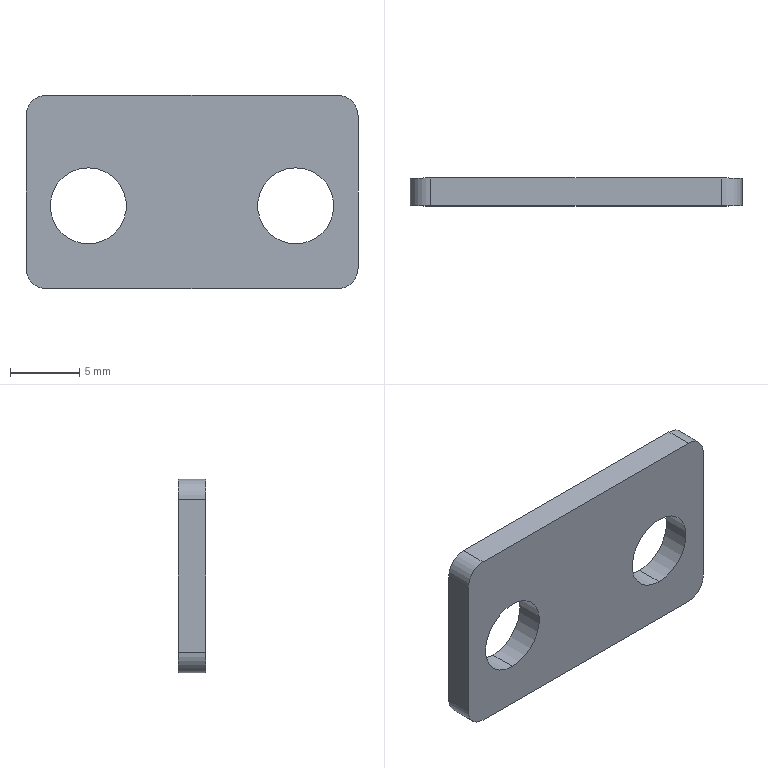Part | STEP file | 0245_011_WSHPK5 | 1 solid | 14 faces | box 24 x 2 x 14 mm | volume 573.104 mm3 | cylinder 8 | plane 6 | commonest cylinder face diameters 3 x4 5.5 x4
STEP:
#1=CARTESIAN_POINT('',(0.,0.,0.));
#2=DIRECTION('',(0.,0.,1.));
#3=DIRECTION('',(1.,0.,0.));
#4=AXIS2_PLACEMENT_3D('',#1,#2,#3);
#5=CARTESIAN_POINT('',(-7.5,2.,-10.75));
#6=VERTEX_POINT('',#5);
#7=CARTESIAN_POINT('',(-7.5,0.,-10.75));
#8=VERTEX_POINT('',#7);
#9=CARTESIAN_POINT('',(-7.5,0.,-10.75));
#10=DIRECTION('',(0.,-1.,0.));
#11=VECTOR('',#10,1.);
#12=LINE('',#9,#11);
#13=CARTESIAN_POINT('',(-7.5,0.,-8.));
#14=DIRECTION('',(0.,-1.,0.));
#15=DIRECTION('',(0.,0.,-1.));
#16=AXIS2_PLACEMENT_3D('',#13,#14,#15);
#17=CYLINDRICAL_SURFACE('',#16,2.75);
#18=CARTESIAN_POINT('',(6.283,0.));
#19=DIRECTION('',(0.,1.));
#20=VECTOR('',#19,1.);
#21=LINE('',#18,#20);
#22=(GEOMETRIC_REPRESENTATION_CONTEXT(2)PARAMETRIC_REPRESENTATION_CONTEXT()REPRESENTATION_CONTEXT('',''));
#23=DEFINITIONAL_REPRESENTATION('',(#21),#22);
#24=PCURVE('',#17,#23);
#25=CARTESIAN_POINT('',(-7.5,0.,-8.));
#26=DIRECTION('',(0.,-1.,0.));
#27=DIRECTION('',(0.,0.,-1.));
#28=AXIS2_PLACEMENT_3D('',#25,#26,#27);
#29=CYLINDRICAL_SURFACE('',#28,2.75);
#30=CARTESIAN_POINT('',(0.,0.));
#31=DIRECTION('',(0.,1.));
#32=VECTOR('',#31,1.);
#33=LINE('',#30,#32);
#34=(GEOMETRIC_REPRESENTATION_CONTEXT(2)PARAMETRIC_REPRESENTATION_CONTEXT()REPRESENTATION_CONTEXT('',''));
#35=DEFINITIONAL_REPRESENTATION('',(#33),#34);
#36=PCURVE('',#29,#35);
#37=SURFACE_CURVE('',#12,(#24,#36),.PCURVE_S1.);
#38=EDGE_CURVE('',#6,#8,#37,.T.);
#39=ORIENTED_EDGE('',*,*,#38,.T.);
#40=CARTESIAN_POINT('',(-7.5,0.,-5.25));
#41=VERTEX_POINT('',#40);
#42=CARTESIAN_POINT('',(-7.5,0.,-8.));
#43=DIRECTION('',(0.,-1.,0.));
#44=DIRECTION('',(0.,0.,-1.));
#45=AXIS2_PLACEMENT_3D('',#42,#43,#44);
#46=CIRCLE('',#45,2.75);
#47=CARTESIAN_POINT('',(0.,0.));
#48=DIRECTION('',(1.,0.));
#49=VECTOR('',#48,1.);
#50=LINE('',#47,#49);
#51=(GEOMETRIC_REPRESENTATION_CONTEXT(2)PARAMETRIC_REPRESENTATION_CONTEXT()REPRESENTATION_CONTEXT('',''));
#52=DEFINITIONAL_REPRESENTATION('',(#50),#51);
#53=PCURVE('',#17,#52);
#54=CARTESIAN_POINT('',(0.,0.,0.));
#55=DIRECTION('',(0.,1.,0.));
#56=DIRECTION('',(0.,0.,1.));
#57=AXIS2_PLACEMENT_3D('',#54,#55,#56);
#58=PLANE('',#57);
#59=CARTESIAN_POINT('',(-10.75,-7.5));
#60=CARTESIAN_POINT('',(-10.75,-2.737));
#61=CARTESIAN_POINT('',(-6.625,-5.118));
#62=CARTESIAN_POINT('',(-2.5,-7.5));
#63=CARTESIAN_POINT('',(-6.625,-9.882));
#64=CARTESIAN_POINT('',(-10.75,-12.263));
#65=CARTESIAN_POINT('',(-10.75,-7.5));
#66=(BOUNDED_CURVE()B_SPLINE_CURVE(2,(#59,#60,#61,#62,#63,#64,#65),.UNSPECIFIED.,.T.,.F.)B_SPLINE_CURVE_WITH_KNOTS((1,2,2,2,2,1),(-2.094,0.,2.094,4.189,6.283,8.378),.UNSPECIFIED.)CURVE()GEOMETRIC_REPRESENTATION_ITEM()RATIONAL_B_SPLINE_CURVE((1.,0.5,1.,0.5,1.,0.5,1.))REPRESENTATION_ITEM(''));
#67=(GEOMETRIC_REPRESENTATION_CONTEXT(2)PARAMETRIC_REPRESENTATION_CONTEXT()REPRESENTATION_CONTEXT('',''));
#68=DEFINITIONAL_REPRESENTATION('',(#66),#67);
#69=PCURVE('',#58,#68);
#70=SURFACE_CURVE('',#46,(#53,#69),.PCURVE_S1.);
#71=EDGE_CURVE('',#41,#8,#70,.T.);
#72=ORIENTED_EDGE('',*,*,#71,.F.);
#73=CARTESIAN_POINT('',(-7.5,2.,-5.25));
#74=VERTEX_POINT('',#73);
#75=CARTESIAN_POINT('',(-7.5,0.,-5.25));
#76=DIRECTION('',(0.,-1.,0.));
#77=VECTOR('',#76,1.);
#78=LINE('',#75,#77);
#79=CARTESIAN_POINT('',(3.142,0.));
#80=DIRECTION('',(0.,1.));
#81=VECTOR('',#80,1.);
#82=LINE('',#79,#81);
#83=(GEOMETRIC_REPRESENTATION_CONTEXT(2)PARAMETRIC_REPRESENTATION_CONTEXT()REPRESENTATION_CONTEXT('',''));
#84=DEFINITIONAL_REPRESENTATION('',(#82),#83);
#85=PCURVE('',#17,#84);
#86=CARTESIAN_POINT('',(3.142,0.));
#87=DIRECTION('',(0.,1.));
#88=VECTOR('',#87,1.);
#89=LINE('',#86,#88);
#90=(GEOMETRIC_REPRESENTATION_CONTEXT(2)PARAMETRIC_REPRESENTATION_CONTEXT()REPRESENTATION_CONTEXT('',''));
#91=DEFINITIONAL_REPRESENTATION('',(#89),#90);
#92=PCURVE('',#29,#91);
#93=SURFACE_CURVE('',#78,(#85,#92),.PCURVE_S1.);
#94=EDGE_CURVE('',#74,#41,#93,.T.);
#95=ORIENTED_EDGE('',*,*,#94,.F.);
#96=CARTESIAN_POINT('',(-7.5,2.,-8.));
#97=DIRECTION('',(0.,-1.,0.));
#98=DIRECTION('',(0.,0.,-1.));
#99=AXIS2_PLACEMENT_3D('',#96,#97,#98);
#100=CIRCLE('',#99,2.75);
#101=CARTESIAN_POINT('',(0.,-2.));
#102=DIRECTION('',(1.,0.));
#103=VECTOR('',#102,1.);
#104=LINE('',#101,#103);
#105=(GEOMETRIC_REPRESENTATION_CONTEXT(2)PARAMETRIC_REPRESENTATION_CONTEXT()REPRESENTATION_CONTEXT('',''));
#106=DEFINITIONAL_REPRESENTATION('',(#104),#105);
#107=PCURVE('',#17,#106);
#108=CARTESIAN_POINT('',(0.,2.,0.));
#109=DIRECTION('',(0.,1.,0.));
#110=DIRECTION('',(0.,0.,1.));
#111=AXIS2_PLACEMENT_3D('',#108,#109,#110);
#112=PLANE('',#111);
#113=CARTESIAN_POINT('',(-10.75,-7.5));
#114=CARTESIAN_POINT('',(-10.75,-2.737));
#115=CARTESIAN_POINT('',(-6.625,-5.118));
#116=CARTESIAN_POINT('',(-2.5,-7.5));
#117=CARTESIAN_POINT('',(-6.625,-9.882));
#118=CARTESIAN_POINT('',(-10.75,-12.263));
#119=CARTESIAN_POINT('',(-10.75,-7.5));
#120=(BOUNDED_CURVE()B_SPLINE_CURVE(2,(#113,#114,#115,#116,#117,#118,#119),.UNSPECIFIED.,.T.,.F.)B_SPLINE_CURVE_WITH_KNOTS((1,2,2,2,2,1),(-2.094,0.,2.094,4.189,6.283,8.378),.UNSPECIFIED.)CURVE()GEOMETRIC_REPRESENTATION_ITEM()RATIONAL_B_SPLINE_CURVE((1.,0.5,1.,0.5,1.,0.5,1.))REPRESENTATION_ITEM(''));
#121=(GEOMETRIC_REPRESENTATION_CONTEXT(2)PARAMETRIC_REPRESENTATION_CONTEXT()REPRESENTATION_CONTEXT('',''));
#122=DEFINITIONAL_REPRESENTATION('',(#120),#121);
#123=PCURVE('',#112,#122);
#124=SURFACE_CURVE('',#100,(#107,#123),.PCURVE_S1.);
#125=EDGE_CURVE('',#74,#6,#124,.T.);
#126=ORIENTED_EDGE('',*,*,#125,.T.);
#127=EDGE_LOOP('',(#39,#72,#95,#126));
#128=FACE_BOUND('',#127,.F.);
#129=ADVANCED_FACE('',(#128),#17,.F.);
#130=CARTESIAN_POINT('',(7.5,2.,-10.75));
#131=VERTEX_POINT('',#130);
#132=CARTESIAN_POINT('',(7.5,0.,-10.75));
#133=VERTEX_POINT('',#132);
#134=CARTESIAN_POINT('',(7.5,0.,-10.75));
#135=DIRECTION('',(0.,-1.,0.));
#136=VECTOR('',#135,1.);
#137=LINE('',#134,#136);
#138=CARTESIAN_POINT('',(7.5,0.,-8.));
#139=DIRECTION('',(0.,-1.,0.));
#140=DIRECTION('',(0.,0.,-1.));
#141=AXIS2_PLACEMENT_3D('',#138,#139,#140);
#142=CYLINDRICAL_SURFACE('',#141,2.75);
#143=CARTESIAN_POINT('',(6.283,0.));
#144=DIRECTION('',(0.,1.));
#145=VECTOR('',#144,1.);
#146=LINE('',#143,#145);
#147=(GEOMETRIC_REPRESENTATION_CONTEXT(2)PARAMETRIC_REPRESENTATION_CONTEXT()REPRESENTATION_CONTEXT('',''));
#148=DEFINITIONAL_REPRESENTATION('',(#146),#147);
#149=PCURVE('',#142,#148);
#150=CARTESIAN_POINT('',(7.5,0.,-8.));
#151=DIRECTION('',(0.,-1.,0.));
#152=DIRECTION('',(0.,0.,-1.));
#153=AXIS2_PLACEMENT_3D('',#150,#151,#152);
#154=CYLINDRICAL_SURFACE('',#153,2.75);
#155=CARTESIAN_POINT('',(0.,0.));
#156=DIRECTION('',(0.,1.));
#157=VECTOR('',#156,1.);
#158=LINE('',#155,#157);
#159=(GEOMETRIC_REPRESENTATION_CONTEXT(2)PARAMETRIC_REPRESENTATION_CONTEXT()REPRESENTATION_CONTEXT('',''));
#160=DEFINITIONAL_REPRESENTATION('',(#158),#159);
#161=PCURVE('',#154,#160);
#162=SURFACE_CURVE('',#137,(#149,#161),.PCURVE_S1.);
#163=EDGE_CURVE('',#131,#133,#162,.T.);
#164=ORIENTED_EDGE('',*,*,#163,.T.);
#165=CARTESIAN_POINT('',(7.5,0.,-5.25));
#166=VERTEX_POINT('',#165);
#167=CARTESIAN_POINT('',(7.5,0.,-8.));
#168=DIRECTION('',(0.,-1.,0.));
#169=DIRECTION('',(0.,0.,-1.));
#170=AXIS2_PLACEMENT_3D('',#167,#168,#169);
#171=CIRCLE('',#170,2.75);
#172=CARTESIAN_POINT('',(0.,0.));
#173=DIRECTION('',(1.,0.));
#174=VECTOR('',#173,1.);
#175=LINE('',#172,#174);
#176=(GEOMETRIC_REPRESENTATION_CONTEXT(2)PARAMETRIC_REPRESENTATION_CONTEXT()REPRESENTATION_CONTEXT('',''));
#177=DEFINITIONAL_REPRESENTATION('',(#175),#176);
#178=PCURVE('',#142,#177);
#179=CARTESIAN_POINT('',(-10.75,7.5));
#180=CARTESIAN_POINT('',(-10.75,12.263));
#181=CARTESIAN_POINT('',(-6.625,9.882));
#182=CARTESIAN_POINT('',(-2.5,7.5));
#183=CARTESIAN_POINT('',(-6.625,5.118));
#184=CARTESIAN_POINT('',(-10.75,2.737));
#185=CARTESIAN_POINT('',(-10.75,7.5));
#186=(BOUNDED_CURVE()B_SPLINE_CURVE(2,(#179,#180,#181,#182,#183,#184,#185),.UNSPECIFIED.,.T.,.F.)B_SPLINE_CURVE_WITH_KNOTS((1,2,2,2,2,1),(-2.094,0.,2.094,4.189,6.283,8.378),.UNSPECIFIED.)CURVE()GEOMETRIC_REPRESENTATION_ITEM()RATIONAL_B_SPLINE_CURVE((1.,0.5,1.,0.5,1.,0.5,1.))REPRESENTATION_ITEM(''));
#187=(GEOMETRIC_REPRESENTATION_CONTEXT(2)PARAMETRIC_REPRESENTATION_CONTEXT()REPRESENTATION_CONTEXT('',''));
#188=DEFINITIONAL_REPRESENTATION('',(#186),#187);
#189=PCURVE('',#58,#188);
#190=SURFACE_CURVE('',#171,(#178,#189),.PCURVE_S1.);
#191=EDGE_CURVE('',#166,#133,#190,.T.);
#192=ORIENTED_EDGE('',*,*,#191,.F.);
#193=CARTESIAN_POINT('',(7.5,2.,-5.25));
#194=VERTEX_POINT('',#193);
#195=CARTESIAN_POINT('',(7.5,0.,-5.25));
#196=DIRECTION('',(0.,-1.,0.));
#197=VECTOR('',#196,1.);
#198=LINE('',#195,#197);
#199=CARTESIAN_POINT('',(3.142,0.));
#200=DIRECTION('',(0.,1.));
#201=VECTOR('',#200,1.);
#202=LINE('',#199,#201);
#203=(GEOMETRIC_REPRESENTATION_CONTEXT(2)PARAMETRIC_REPRESENTATION_CONTEXT()REPRESENTATION_CONTEXT('',''));
#204=DEFINITIONAL_REPRESENTATION('',(#202),#203);
#205=PCURVE('',#142,#204);
#206=CARTESIAN_POINT('',(3.142,0.));
#207=DIRECTION('',(0.,1.));
#208=VECTOR('',#207,1.);
#209=LINE('',#206,#208);
#210=(GEOMETRIC_REPRESENTATION_CONTEXT(2)PARAMETRIC_REPRESENTATION_CONTEXT()REPRESENTATION_CONTEXT('',''));
#211=DEFINITIONAL_REPRESENTATION('',(#209),#210);
#212=PCURVE('',#154,#211);
#213=SURFACE_CURVE('',#198,(#205,#212),.PCURVE_S1.);
#214=EDGE_CURVE('',#194,#166,#213,.T.);
#215=ORIENTED_EDGE('',*,*,#214,.F.);
#216=CARTESIAN_POINT('',(7.5,2.,-8.));
#217=DIRECTION('',(0.,-1.,0.));
#218=DIRECTION('',(0.,0.,-1.));
#219=AXIS2_PLACEMENT_3D('',#216,#217,#218);
#220=CIRCLE('',#219,2.75);
#221=CARTESIAN_POINT('',(0.,-2.));
#222=DIRECTION('',(1.,0.));
#223=VECTOR('',#222,1.);
#224=LINE('',#221,#223);
#225=(GEOMETRIC_REPRESENTATION_CONTEXT(2)PARAMETRIC_REPRESENTATION_CONTEXT()REPRESENTATION_CONTEXT('',''));
#226=DEFINITIONAL_REPRESENTATION('',(#224),#225);
#227=PCURVE('',#142,#226);
#228=CARTESIAN_POINT('',(-10.75,7.5));
#229=CARTESIAN_POINT('',(-10.75,12.263));
#230=CARTESIAN_POINT('',(-6.625,9.882));
#231=CARTESIAN_POINT('',(-2.5,7.5));
#232=CARTESIAN_POINT('',(-6.625,5.118));
#233=CARTESIAN_POINT('',(-10.75,2.737));
#234=CARTESIAN_POINT('',(-10.75,7.5));
#235=(BOUNDED_CURVE()B_SPLINE_CURVE(2,(#228,#229,#230,#231,#232,#233,#234),.UNSPECIFIED.,.T.,.F.)B_SPLINE_CURVE_WITH_KNOTS((1,2,2,2,2,1),(-2.094,0.,2.094,4.189,6.283,8.378),.UNSPECIFIED.)CURVE()GEOMETRIC_REPRESENTATION_ITEM()RATIONAL_B_SPLINE_CURVE((1.,0.5,1.,0.5,1.,0.5,1.))REPRESENTATION_ITEM(''));
#236=(GEOMETRIC_REPRESENTATION_CONTEXT(2)PARAMETRIC_REPRESENTATION_CONTEXT()REPRESENTATION_CONTEXT('',''));
#237=DEFINITIONAL_REPRESENTATION('',(#235),#236);
#238=PCURVE('',#112,#237);
#239=SURFACE_CURVE('',#220,(#227,#238),.PCURVE_S1.);
#240=EDGE_CURVE('',#194,#131,#239,.T.);
#241=ORIENTED_EDGE('',*,*,#240,.T.);
#242=EDGE_LOOP('',(#164,#192,#215,#241));
#243=FACE_BOUND('',#242,.F.);
#244=ADVANCED_FACE('',(#243),#142,.F.);
#245=CARTESIAN_POINT('',(-7.5,0.,-8.));
#246=DIRECTION('',(0.,-1.,0.));
#247=DIRECTION('',(0.,0.,-1.));
#248=AXIS2_PLACEMENT_3D('',#245,#246,#247);
#249=CIRCLE('',#248,2.75);
#250=CARTESIAN_POINT('',(-10.75,-7.5));
#251=CARTESIAN_POINT('',(-10.75,-2.737));
#252=CARTESIAN_POINT('',(-6.625,-5.118));
#253=CARTESIAN_POINT('',(-2.5,-7.5));
#254=CARTESIAN_POINT('',(-6.625,-9.882));
#255=CARTESIAN_POINT('',(-10.75,-12.263));
#256=CARTESIAN_POINT('',(-10.75,-7.5));
#257=(BOUNDED_CURVE()B_SPLINE_CURVE(2,(#250,#251,#252,#253,#254,#255,#256),.UNSPECIFIED.,.T.,.F.)B_SPLINE_CURVE_WITH_KNOTS((1,2,2,2,2,1),(-2.094,0.,2.094,4.189,6.283,8.378),.UNSPECIFIED.)CURVE()GEOMETRIC_REPRESENTATION_ITEM()RATIONAL_B_SPLINE_CURVE((1.,0.5,1.,0.5,1.,0.5,1.))REPRESENTATION_ITEM(''));
#258=(GEOMETRIC_REPRESENTATION_CONTEXT(2)PARAMETRIC_REPRESENTATION_CONTEXT()REPRESENTATION_CONTEXT('',''));
#259=DEFINITIONAL_REPRESENTATION('',(#257),#258);
#260=PCURVE('',#58,#259);
#261=CARTESIAN_POINT('',(0.,0.));
#262=DIRECTION('',(1.,0.));
#263=VECTOR('',#262,1.);
#264=LINE('',#261,#263);
#265=(GEOMETRIC_REPRESENTATION_CONTEXT(2)PARAMETRIC_REPRESENTATION_CONTEXT()REPRESENTATION_CONTEXT('',''));
#266=DEFINITIONAL_REPRESENTATION('',(#264),#265);
#267=PCURVE('',#29,#266);
#268=SURFACE_CURVE('',#249,(#260,#267),.PCURVE_S1.);
#269=EDGE_CURVE('',#8,#41,#268,.T.);
#270=ORIENTED_EDGE('',*,*,#269,.F.);
#271=ORIENTED_EDGE('',*,*,#71,.F.);
#272=EDGE_LOOP('',(#270,#271));
#273=FACE_BOUND('',#272,.T.);
#274=CARTESIAN_POINT('',(7.5,0.,-8.));
#275=DIRECTION('',(0.,-1.,0.));
#276=DIRECTION('',(0.,0.,-1.));
#277=AXIS2_PLACEMENT_3D('',#274,#275,#276);
#278=CIRCLE('',#277,2.75);
#279=CARTESIAN_POINT('',(-10.75,7.5));
#280=CARTESIAN_POINT('',(-10.75,12.263));
#281=CARTESIAN_POINT('',(-6.625,9.882));
#282=CARTESIAN_POINT('',(-2.5,7.5));
#283=CARTESIAN_POINT('',(-6.625,5.118));
#284=CARTESIAN_POINT('',(-10.75,2.737));
#285=CARTESIAN_POINT('',(-10.75,7.5));
#286=(BOUNDED_CURVE()B_SPLINE_CURVE(2,(#279,#280,#281,#282,#283,#284,#285),.UNSPECIFIED.,.T.,.F.)B_SPLINE_CURVE_WITH_KNOTS((1,2,2,2,2,1),(-2.094,0.,2.094,4.189,6.283,8.378),.UNSPECIFIED.)CURVE()GEOMETRIC_REPRESENTATION_ITEM()RATIONAL_B_SPLINE_CURVE((1.,0.5,1.,0.5,1.,0.5,1.))REPRESENTATION_ITEM(''));
#287=(GEOMETRIC_REPRESENTATION_CONTEXT(2)PARAMETRIC_REPRESENTATION_CONTEXT()REPRESENTATION_CONTEXT('',''));
#288=DEFINITIONAL_REPRESENTATION('',(#286),#287);
#289=PCURVE('',#58,#288);
#290=CARTESIAN_POINT('',(0.,0.));
#291=DIRECTION('',(1.,0.));
#292=VECTOR('',#291,1.);
#293=LINE('',#290,#292);
#294=(GEOMETRIC_REPRESENTATION_CONTEXT(2)PARAMETRIC_REPRESENTATION_CONTEXT()REPRESENTATION_CONTEXT('',''));
#295=DEFINITIONAL_REPRESENTATION('',(#293),#294);
#296=PCURVE('',#154,#295);
#297=SURFACE_CURVE('',#278,(#289,#296),.PCURVE_S1.);
#298=EDGE_CURVE('',#133,#166,#297,.T.);
#299=ORIENTED_EDGE('',*,*,#298,.F.);
#300=ORIENTED_EDGE('',*,*,#191,.F.);
#301=EDGE_LOOP('',(#299,#300));
#302=FACE_BOUND('',#301,.T.);
#303=CARTESIAN_POINT('',(-10.5,0.,-14.));
#304=VERTEX_POINT('',#303);
#305=CARTESIAN_POINT('',(-12.,0.,-12.5));
#306=VERTEX_POINT('',#305);
#307=CARTESIAN_POINT('',(-10.5,0.,-12.5));
#308=DIRECTION('',(0.,1.,0.));
#309=DIRECTION('',(0.,0.,-1.));
#310=AXIS2_PLACEMENT_3D('',#307,#308,#309);
#311=CIRCLE('',#310,1.5);
#312=CARTESIAN_POINT('',(-12.5,-10.5));
#313=DIRECTION('',(-1.,0.));
#314=AXIS2_PLACEMENT_2D('',#312,#313);
#315=CIRCLE('',#314,1.5);
#316=(GEOMETRIC_REPRESENTATION_CONTEXT(2)PARAMETRIC_REPRESENTATION_CONTEXT()REPRESENTATION_CONTEXT('',''));
#317=DEFINITIONAL_REPRESENTATION('',(#315),#316);
#318=PCURVE('',#58,#317);
#319=CARTESIAN_POINT('',(-10.5,0.,-12.5));
#320=DIRECTION('',(0.,-1.,0.));
#321=DIRECTION('',(0.,0.,-1.));
#322=AXIS2_PLACEMENT_3D('',#319,#320,#321);
#323=CYLINDRICAL_SURFACE('',#322,1.5);
#324=CARTESIAN_POINT('',(6.283,0.));
#325=DIRECTION('',(-1.,0.));
#326=VECTOR('',#325,1.);
#327=LINE('',#324,#326);
#328=(GEOMETRIC_REPRESENTATION_CONTEXT(2)PARAMETRIC_REPRESENTATION_CONTEXT()REPRESENTATION_CONTEXT('',''));
#329=DEFINITIONAL_REPRESENTATION('',(#327),#328);
#330=PCURVE('',#323,#329);
#331=SURFACE_CURVE('',#311,(#318,#330),.PCURVE_S1.);
#332=EDGE_CURVE('',#304,#306,#331,.T.);
#333=ORIENTED_EDGE('',*,*,#332,.F.);
#334=CARTESIAN_POINT('',(10.5,0.,-14.));
#335=VERTEX_POINT('',#334);
#336=CARTESIAN_POINT('',(0.,0.,-14.));
#337=DIRECTION('',(-1.,0.,0.));
#338=VECTOR('',#337,1.);
#339=LINE('',#336,#338);
#340=CARTESIAN_POINT('',(-14.,0.));
#341=DIRECTION('',(0.,-1.));
#342=VECTOR('',#341,1.);
#343=LINE('',#340,#342);
#344=(GEOMETRIC_REPRESENTATION_CONTEXT(2)PARAMETRIC_REPRESENTATION_CONTEXT()REPRESENTATION_CONTEXT('',''));
#345=DEFINITIONAL_REPRESENTATION('',(#343),#344);
#346=PCURVE('',#58,#345);
#347=CARTESIAN_POINT('',(-10.5,0.,-14.));
#348=DIRECTION('',(0.,0.,-1.));
#349=DIRECTION('',(-1.,0.,0.));
#350=AXIS2_PLACEMENT_3D('',#347,#348,#349);
#351=PLANE('',#350);
#352=CARTESIAN_POINT('',(-10.5,0.));
#353=DIRECTION('',(1.,0.));
#354=VECTOR('',#353,1.);
#355=LINE('',#352,#354);
#356=(GEOMETRIC_REPRESENTATION_CONTEXT(2)PARAMETRIC_REPRESENTATION_CONTEXT()REPRESENTATION_CONTEXT('',''));
#357=DEFINITIONAL_REPRESENTATION('',(#355),#356);
#358=PCURVE('',#351,#357);
#359=SURFACE_CURVE('',#339,(#346,#358),.PCURVE_S1.);
#360=EDGE_CURVE('',#335,#304,#359,.T.);
#361=ORIENTED_EDGE('',*,*,#360,.F.);
#362=CARTESIAN_POINT('',(12.,0.,-12.5));
#363=VERTEX_POINT('',#362);
#364=CARTESIAN_POINT('',(10.5,0.,-12.5));
#365=DIRECTION('',(0.,1.,0.));
#366=DIRECTION('',(0.,0.,-1.));
#367=AXIS2_PLACEMENT_3D('',#364,#365,#366);
#368=CIRCLE('',#367,1.5);
#369=CARTESIAN_POINT('',(-12.5,10.5));
#370=DIRECTION('',(-1.,0.));
#371=AXIS2_PLACEMENT_2D('',#369,#370);
#372=CIRCLE('',#371,1.5);
#373=(GEOMETRIC_REPRESENTATION_CONTEXT(2)PARAMETRIC_REPRESENTATION_CONTEXT()REPRESENTATION_CONTEXT('',''));
#374=DEFINITIONAL_REPRESENTATION('',(#372),#373);
#375=PCURVE('',#58,#374);
#376=CARTESIAN_POINT('',(10.5,0.,-12.5));
#377=DIRECTION('',(0.,-1.,0.));
#378=DIRECTION('',(0.,0.,-1.));
#379=AXIS2_PLACEMENT_3D('',#376,#377,#378);
#380=CYLINDRICAL_SURFACE('',#379,1.5);
#381=CARTESIAN_POINT('',(6.283,0.));
#382=DIRECTION('',(-1.,0.));
#383=VECTOR('',#382,1.);
#384=LINE('',#381,#383);
#385=(GEOMETRIC_REPRESENTATION_CONTEXT(2)PARAMETRIC_REPRESENTATION_CONTEXT()REPRESENTATION_CONTEXT('',''));
#386=DEFINITIONAL_REPRESENTATION('',(#384),#385);
#387=PCURVE('',#380,#386);
#388=SURFACE_CURVE('',#368,(#375,#387),.PCURVE_S1.);
#389=EDGE_CURVE('',#363,#335,#388,.T.);
#390=ORIENTED_EDGE('',*,*,#389,.F.);
#391=CARTESIAN_POINT('',(12.,0.,-1.5));
#392=VERTEX_POINT('',#391);
#393=CARTESIAN_POINT('',(12.,0.,0.));
#394=DIRECTION('',(0.,0.,-1.));
#395=VECTOR('',#394,1.);
#396=LINE('',#393,#395);
#397=CARTESIAN_POINT('',(0.,12.));
#398=DIRECTION('',(-1.,0.));
#399=VECTOR('',#398,1.);
#400=LINE('',#397,#399);
#401=(GEOMETRIC_REPRESENTATION_CONTEXT(2)PARAMETRIC_REPRESENTATION_CONTEXT()REPRESENTATION_CONTEXT('',''));
#402=DEFINITIONAL_REPRESENTATION('',(#400),#401);
#403=PCURVE('',#58,#402);
#404=CARTESIAN_POINT('',(12.,0.,-12.5));
#405=DIRECTION('',(1.,0.,0.));
#406=DIRECTION('',(0.,0.,-1.));
#407=AXIS2_PLACEMENT_3D('',#404,#405,#406);
#408=PLANE('',#407);
#409=CARTESIAN_POINT('',(-12.5,0.));
#410=DIRECTION('',(1.,0.));
#411=VECTOR('',#410,1.);
#412=LINE('',#409,#411);
#413=(GEOMETRIC_REPRESENTATION_CONTEXT(2)PARAMETRIC_REPRESENTATION_CONTEXT()REPRESENTATION_CONTEXT('',''));
#414=DEFINITIONAL_REPRESENTATION('',(#412),#413);
#415=PCURVE('',#408,#414);
#416=SURFACE_CURVE('',#396,(#403,#415),.PCURVE_S1.);
#417=EDGE_CURVE('',#392,#363,#416,.T.);
#418=ORIENTED_EDGE('',*,*,#417,.F.);
#419=CARTESIAN_POINT('',(10.5,0.,0.));
#420=VERTEX_POINT('',#419);
#421=CARTESIAN_POINT('',(10.5,0.,-1.5));
#422=DIRECTION('',(0.,1.,0.));
#423=DIRECTION('',(0.,0.,-1.));
#424=AXIS2_PLACEMENT_3D('',#421,#422,#423);
#425=CIRCLE('',#424,1.5);
#426=CARTESIAN_POINT('',(-1.5,10.5));
#427=DIRECTION('',(-1.,0.));
#428=AXIS2_PLACEMENT_2D('',#426,#427);
#429=CIRCLE('',#428,1.5);
#430=(GEOMETRIC_REPRESENTATION_CONTEXT(2)PARAMETRIC_REPRESENTATION_CONTEXT()REPRESENTATION_CONTEXT('',''));
#431=DEFINITIONAL_REPRESENTATION('',(#429),#430);
#432=PCURVE('',#58,#431);
#433=CARTESIAN_POINT('',(10.5,0.,-1.5));
#434=DIRECTION('',(0.,-1.,0.));
#435=DIRECTION('',(0.,0.,-1.));
#436=AXIS2_PLACEMENT_3D('',#433,#434,#435);
#437=CYLINDRICAL_SURFACE('',#436,1.5);
#438=CARTESIAN_POINT('',(6.283,0.));
#439=DIRECTION('',(-1.,0.));
#440=VECTOR('',#439,1.);
#441=LINE('',#438,#440);
#442=(GEOMETRIC_REPRESENTATION_CONTEXT(2)PARAMETRIC_REPRESENTATION_CONTEXT()REPRESENTATION_CONTEXT('',''));
#443=DEFINITIONAL_REPRESENTATION('',(#441),#442);
#444=PCURVE('',#437,#443);
#445=SURFACE_CURVE('',#425,(#432,#444),.PCURVE_S1.);
#446=EDGE_CURVE('',#420,#392,#445,.T.);
#447=ORIENTED_EDGE('',*,*,#446,.F.);
#448=CARTESIAN_POINT('',(-10.5,0.,0.));
#449=VERTEX_POINT('',#448);
#450=CARTESIAN_POINT('',(0.,0.,0.));
#451=DIRECTION('',(1.,0.,0.));
#452=VECTOR('',#451,1.);
#453=LINE('',#450,#452);
#454=CARTESIAN_POINT('',(0.,0.));
#455=DIRECTION('',(0.,1.));
#456=VECTOR('',#455,1.);
#457=LINE('',#454,#456);
#458=(GEOMETRIC_REPRESENTATION_CONTEXT(2)PARAMETRIC_REPRESENTATION_CONTEXT()REPRESENTATION_CONTEXT('',''));
#459=DEFINITIONAL_REPRESENTATION('',(#457),#458);
#460=PCURVE('',#58,#459);
#461=CARTESIAN_POINT('',(10.5,0.,0.));
#462=DIRECTION('',(0.,0.,1.));
#463=DIRECTION('',(1.,0.,0.));
#464=AXIS2_PLACEMENT_3D('',#461,#462,#463);
#465=PLANE('',#464);
#466=CARTESIAN_POINT('',(-10.5,0.));
#467=DIRECTION('',(1.,0.));
#468=VECTOR('',#467,1.);
#469=LINE('',#466,#468);
#470=(GEOMETRIC_REPRESENTATION_CONTEXT(2)PARAMETRIC_REPRESENTATION_CONTEXT()REPRESENTATION_CONTEXT('',''));
#471=DEFINITIONAL_REPRESENTATION('',(#469),#470);
#472=PCURVE('',#465,#471);
#473=SURFACE_CURVE('',#453,(#460,#472),.PCURVE_S1.);
#474=EDGE_CURVE('',#449,#420,#473,.T.);
#475=ORIENTED_EDGE('',*,*,#474,.F.);
#476=CARTESIAN_POINT('',(-12.,0.,-1.5));
#477=VERTEX_POINT('',#476);
#478=CARTESIAN_POINT('',(-10.5,0.,-1.5));
#479=DIRECTION('',(0.,1.,0.));
#480=DIRECTION('',(0.,0.,-1.));
#481=AXIS2_PLACEMENT_3D('',#478,#479,#480);
#482=CIRCLE('',#481,1.5);
#483=CARTESIAN_POINT('',(-1.5,-10.5));
#484=DIRECTION('',(-1.,0.));
#485=AXIS2_PLACEMENT_2D('',#483,#484);
#486=CIRCLE('',#485,1.5);
#487=(GEOMETRIC_REPRESENTATION_CONTEXT(2)PARAMETRIC_REPRESENTATION_CONTEXT()REPRESENTATION_CONTEXT('',''));
#488=DEFINITIONAL_REPRESENTATION('',(#486),#487);
#489=PCURVE('',#58,#488);
#490=CARTESIAN_POINT('',(-10.5,0.,-1.5));
#491=DIRECTION('',(0.,-1.,0.));
#492=DIRECTION('',(0.,0.,-1.));
#493=AXIS2_PLACEMENT_3D('',#490,#491,#492);
#494=CYLINDRICAL_SURFACE('',#493,1.5);
#495=CARTESIAN_POINT('',(6.283,0.));
#496=DIRECTION('',(-1.,0.));
#497=VECTOR('',#496,1.);
#498=LINE('',#495,#497);
#499=(GEOMETRIC_REPRESENTATION_CONTEXT(2)PARAMETRIC_REPRESENTATION_CONTEXT()REPRESENTATION_CONTEXT('',''));
#500=DEFINITIONAL_REPRESENTATION('',(#498),#499);
#501=PCURVE('',#494,#500);
#502=SURFACE_CURVE('',#482,(#489,#501),.PCURVE_S1.);
#503=EDGE_CURVE('',#477,#449,#502,.T.);
#504=ORIENTED_EDGE('',*,*,#503,.F.);
#505=CARTESIAN_POINT('',(-12.,0.,0.));
#506=DIRECTION('',(0.,0.,1.));
#507=VECTOR('',#506,1.);
#508=LINE('',#505,#507);
#509=CARTESIAN_POINT('',(0.,-12.));
#510=DIRECTION('',(1.,0.));
#511=VECTOR('',#510,1.);
#512=LINE('',#509,#511);
#513=(GEOMETRIC_REPRESENTATION_CONTEXT(2)PARAMETRIC_REPRESENTATION_CONTEXT()REPRESENTATION_CONTEXT('',''));
#514=DEFINITIONAL_REPRESENTATION('',(#512),#513);
#515=PCURVE('',#58,#514);
#516=CARTESIAN_POINT('',(-12.,0.,-1.5));
#517=DIRECTION('',(-1.,0.,0.));
#518=DIRECTION('',(0.,0.,1.));
#519=AXIS2_PLACEMENT_3D('',#516,#517,#518);
#520=PLANE('',#519);
#521=CARTESIAN_POINT('',(1.5,0.));
#522=DIRECTION('',(1.,0.));
#523=VECTOR('',#522,1.);
#524=LINE('',#521,#523);
#525=(GEOMETRIC_REPRESENTATION_CONTEXT(2)PARAMETRIC_REPRESENTATION_CONTEXT()REPRESENTATION_CONTEXT('',''));
#526=DEFINITIONAL_REPRESENTATION('',(#524),#525);
#527=PCURVE('',#520,#526);
#528=SURFACE_CURVE('',#508,(#515,#527),.PCURVE_S1.);
#529=EDGE_CURVE('',#306,#477,#528,.T.);
#530=ORIENTED_EDGE('',*,*,#529,.F.);
#531=EDGE_LOOP('',(#333,#361,#390,#418,#447,#475,#504,#530));
#532=FACE_BOUND('',#531,.T.);
#533=ADVANCED_FACE('',(#273,#302,#532),#58,.F.);
#534=ORIENTED_EDGE('',*,*,#269,.F.);
#535=ORIENTED_EDGE('',*,*,#38,.F.);
#536=CARTESIAN_POINT('',(-7.5,2.,-8.));
#537=DIRECTION('',(0.,-1.,0.));
#538=DIRECTION('',(0.,0.,-1.));
#539=AXIS2_PLACEMENT_3D('',#536,#537,#538);
#540=CIRCLE('',#539,2.75);
#541=CARTESIAN_POINT('',(0.,-2.));
#542=DIRECTION('',(1.,0.));
#543=VECTOR('',#542,1.);
#544=LINE('',#541,#543);
#545=(GEOMETRIC_REPRESENTATION_CONTEXT(2)PARAMETRIC_REPRESENTATION_CONTEXT()REPRESENTATION_CONTEXT('',''));
#546=DEFINITIONAL_REPRESENTATION('',(#544),#545);
#547=PCURVE('',#29,#546);
#548=CARTESIAN_POINT('',(-10.75,-7.5));
#549=CARTESIAN_POINT('',(-10.75,-2.737));
#550=CARTESIAN_POINT('',(-6.625,-5.118));
#551=CARTESIAN_POINT('',(-2.5,-7.5));
#552=CARTESIAN_POINT('',(-6.625,-9.882));
#553=CARTESIAN_POINT('',(-10.75,-12.263));
#554=CARTESIAN_POINT('',(-10.75,-7.5));
#555=(BOUNDED_CURVE()B_SPLINE_CURVE(2,(#548,#549,#550,#551,#552,#553,#554),.UNSPECIFIED.,.T.,.F.)B_SPLINE_CURVE_WITH_KNOTS((1,2,2,2,2,1),(-2.094,0.,2.094,4.189,6.283,8.378),.UNSPECIFIED.)CURVE()GEOMETRIC_REPRESENTATION_ITEM()RATIONAL_B_SPLINE_CURVE((1.,0.5,1.,0.5,1.,0.5,1.))REPRESENTATION_ITEM(''));
#556=(GEOMETRIC_REPRESENTATION_CONTEXT(2)PARAMETRIC_REPRESENTATION_CONTEXT()REPRESENTATION_CONTEXT('',''));
#557=DEFINITIONAL_REPRESENTATION('',(#555),#556);
#558=PCURVE('',#112,#557);
#559=SURFACE_CURVE('',#540,(#547,#558),.PCURVE_S1.);
#560=EDGE_CURVE('',#6,#74,#559,.T.);
#561=ORIENTED_EDGE('',*,*,#560,.T.);
#562=ORIENTED_EDGE('',*,*,#94,.T.);
#563=EDGE_LOOP('',(#534,#535,#561,#562));
#564=FACE_BOUND('',#563,.F.);
#565=ADVANCED_FACE('',(#564),#29,.F.);
#566=ORIENTED_EDGE('',*,*,#298,.F.);
#567=ORIENTED_EDGE('',*,*,#163,.F.);
#568=CARTESIAN_POINT('',(7.5,2.,-8.));
#569=DIRECTION('',(0.,-1.,0.));
#570=DIRECTION('',(0.,0.,-1.));
#571=AXIS2_PLACEMENT_3D('',#568,#569,#570);
#572=CIRCLE('',#571,2.75);
#573=CARTESIAN_POINT('',(0.,-2.));
#574=DIRECTION('',(1.,0.));
#575=VECTOR('',#574,1.);
#576=LINE('',#573,#575);
#577=(GEOMETRIC_REPRESENTATION_CONTEXT(2)PARAMETRIC_REPRESENTATION_CONTEXT()REPRESENTATION_CONTEXT('',''));
#578=DEFINITIONAL_REPRESENTATION('',(#576),#577);
#579=PCURVE('',#154,#578);
#580=CARTESIAN_POINT('',(-10.75,7.5));
#581=CARTESIAN_POINT('',(-10.75,12.263));
#582=CARTESIAN_POINT('',(-6.625,9.882));
#583=CARTESIAN_POINT('',(-2.5,7.5));
#584=CARTESIAN_POINT('',(-6.625,5.118));
#585=CARTESIAN_POINT('',(-10.75,2.737));
#586=CARTESIAN_POINT('',(-10.75,7.5));
#587=(BOUNDED_CURVE()B_SPLINE_CURVE(2,(#580,#581,#582,#583,#584,#585,#586),.UNSPECIFIED.,.T.,.F.)B_SPLINE_CURVE_WITH_KNOTS((1,2,2,2,2,1),(-2.094,0.,2.094,4.189,6.283,8.378),.UNSPECIFIED.)CURVE()GEOMETRIC_REPRESENTATION_ITEM()RATIONAL_B_SPLINE_CURVE((1.,0.5,1.,0.5,1.,0.5,1.))REPRESENTATION_ITEM(''));
#588=(GEOMETRIC_REPRESENTATION_CONTEXT(2)PARAMETRIC_REPRESENTATION_CONTEXT()REPRESENTATION_CONTEXT('',''));
#589=DEFINITIONAL_REPRESENTATION('',(#587),#588);
#590=PCURVE('',#112,#589);
#591=SURFACE_CURVE('',#572,(#579,#590),.PCURVE_S1.);
#592=EDGE_CURVE('',#131,#194,#591,.T.);
#593=ORIENTED_EDGE('',*,*,#592,.T.);
#594=ORIENTED_EDGE('',*,*,#214,.T.);
#595=EDGE_LOOP('',(#566,#567,#593,#594));
#596=FACE_BOUND('',#595,.F.);
#597=ADVANCED_FACE('',(#596),#154,.F.);
#598=ORIENTED_EDGE('',*,*,#529,.T.);
#599=CARTESIAN_POINT('',(-12.,2.,-1.5));
#600=VERTEX_POINT('',#599);
#601=CARTESIAN_POINT('',(-12.,0.,-1.5));
#602=DIRECTION('',(0.,1.,0.));
#603=VECTOR('',#602,1.);
#604=LINE('',#601,#603);
#605=CARTESIAN_POINT('',(0.,0.));
#606=DIRECTION('',(0.,1.));
#607=VECTOR('',#606,1.);
#608=LINE('',#605,#607);
#609=(GEOMETRIC_REPRESENTATION_CONTEXT(2)PARAMETRIC_REPRESENTATION_CONTEXT()REPRESENTATION_CONTEXT('',''));
#610=DEFINITIONAL_REPRESENTATION('',(#608),#609);
#611=PCURVE('',#520,#610);
#612=CARTESIAN_POINT('',(4.712,0.));
#613=DIRECTION('',(0.,-1.));
#614=VECTOR('',#613,1.);
#615=LINE('',#612,#614);
#616=(GEOMETRIC_REPRESENTATION_CONTEXT(2)PARAMETRIC_REPRESENTATION_CONTEXT()REPRESENTATION_CONTEXT('',''));
#617=DEFINITIONAL_REPRESENTATION('',(#615),#616);
#618=PCURVE('',#494,#617);
#619=SURFACE_CURVE('',#604,(#611,#618),.PCURVE_S1.);
#620=EDGE_CURVE('',#477,#600,#619,.T.);
#621=ORIENTED_EDGE('',*,*,#620,.T.);
#622=CARTESIAN_POINT('',(-12.,2.,-12.5));
#623=VERTEX_POINT('',#622);
#624=CARTESIAN_POINT('',(-12.,2.,-1.5));
#625=DIRECTION('',(0.,0.,-1.));
#626=VECTOR('',#625,1.);
#627=LINE('',#624,#626);
#628=CARTESIAN_POINT('',(0.,2.));
#629=DIRECTION('',(-1.,0.));
#630=VECTOR('',#629,1.);
#631=LINE('',#628,#630);
#632=(GEOMETRIC_REPRESENTATION_CONTEXT(2)PARAMETRIC_REPRESENTATION_CONTEXT()REPRESENTATION_CONTEXT('',''));
#633=DEFINITIONAL_REPRESENTATION('',(#631),#632);
#634=PCURVE('',#520,#633);
#635=CARTESIAN_POINT('',(-1.5,-12.));
#636=DIRECTION('',(-1.,0.));
#637=VECTOR('',#636,1.);
#638=LINE('',#635,#637);
#639=(GEOMETRIC_REPRESENTATION_CONTEXT(2)PARAMETRIC_REPRESENTATION_CONTEXT()REPRESENTATION_CONTEXT('',''));
#640=DEFINITIONAL_REPRESENTATION('',(#638),#639);
#641=PCURVE('',#112,#640);
#642=SURFACE_CURVE('',#627,(#634,#641),.PCURVE_S1.);
#643=EDGE_CURVE('',#600,#623,#642,.T.);
#644=ORIENTED_EDGE('',*,*,#643,.T.);
#645=CARTESIAN_POINT('',(-12.,0.,-12.5));
#646=DIRECTION('',(0.,-1.,0.));
#647=VECTOR('',#646,1.);
#648=LINE('',#645,#647);
#649=CARTESIAN_POINT('',(-11.,0.));
#650=DIRECTION('',(0.,-1.));
#651=VECTOR('',#650,1.);
#652=LINE('',#649,#651);
#653=(GEOMETRIC_REPRESENTATION_CONTEXT(2)PARAMETRIC_REPRESENTATION_CONTEXT()REPRESENTATION_CONTEXT('',''));
#654=DEFINITIONAL_REPRESENTATION('',(#652),#653);
#655=PCURVE('',#520,#654);
#656=CARTESIAN_POINT('',(4.712,0.));
#657=DIRECTION('',(0.,1.));
#658=VECTOR('',#657,1.);
#659=LINE('',#656,#658);
#660=(GEOMETRIC_REPRESENTATION_CONTEXT(2)PARAMETRIC_REPRESENTATION_CONTEXT()REPRESENTATION_CONTEXT('',''));
#661=DEFINITIONAL_REPRESENTATION('',(#659),#660);
#662=PCURVE('',#323,#661);
#663=SURFACE_CURVE('',#648,(#655,#662),.PCURVE_S1.);
#664=EDGE_CURVE('',#623,#306,#663,.T.);
#665=ORIENTED_EDGE('',*,*,#664,.T.);
#666=EDGE_LOOP('',(#598,#621,#644,#665));
#667=FACE_BOUND('',#666,.T.);
#668=ADVANCED_FACE('',(#667),#520,.T.);
#669=ORIENTED_EDGE('',*,*,#332,.T.);
#670=ORIENTED_EDGE('',*,*,#664,.F.);
#671=CARTESIAN_POINT('',(-10.5,2.,-14.));
#672=VERTEX_POINT('',#671);
#673=CARTESIAN_POINT('',(-10.5,2.,-12.5));
#674=DIRECTION('',(0.,-1.,0.));
#675=DIRECTION('',(0.,0.,-1.));
#676=AXIS2_PLACEMENT_3D('',#673,#674,#675);
#677=CIRCLE('',#676,1.5);
#678=CARTESIAN_POINT('',(0.,-2.));
#679=DIRECTION('',(1.,0.));
#680=VECTOR('',#679,1.);
#681=LINE('',#678,#680);
#682=(GEOMETRIC_REPRESENTATION_CONTEXT(2)PARAMETRIC_REPRESENTATION_CONTEXT()REPRESENTATION_CONTEXT('',''));
#683=DEFINITIONAL_REPRESENTATION('',(#681),#682);
#684=PCURVE('',#323,#683);
#685=CARTESIAN_POINT('',(-14.,-10.5));
#686=CARTESIAN_POINT('',(-14.,-7.902));
#687=CARTESIAN_POINT('',(-11.75,-9.201));
#688=CARTESIAN_POINT('',(-9.5,-10.5));
#689=CARTESIAN_POINT('',(-11.75,-11.799));
#690=CARTESIAN_POINT('',(-14.,-13.098));
#691=CARTESIAN_POINT('',(-14.,-10.5));
#692=(BOUNDED_CURVE()B_SPLINE_CURVE(2,(#685,#686,#687,#688,#689,#690,#691),.UNSPECIFIED.,.T.,.F.)B_SPLINE_CURVE_WITH_KNOTS((1,2,2,2,2,1),(-2.094,0.,2.094,4.189,6.283,8.378),.UNSPECIFIED.)CURVE()GEOMETRIC_REPRESENTATION_ITEM()RATIONAL_B_SPLINE_CURVE((1.,0.5,1.,0.5,1.,0.5,1.))REPRESENTATION_ITEM(''));
#693=(GEOMETRIC_REPRESENTATION_CONTEXT(2)PARAMETRIC_REPRESENTATION_CONTEXT()REPRESENTATION_CONTEXT('',''));
#694=DEFINITIONAL_REPRESENTATION('',(#692),#693);
#695=PCURVE('',#112,#694);
#696=SURFACE_CURVE('',#677,(#684,#695),.PCURVE_S1.);
#697=EDGE_CURVE('',#623,#672,#696,.T.);
#698=ORIENTED_EDGE('',*,*,#697,.T.);
#699=CARTESIAN_POINT('',(-10.5,0.,-14.));
#700=DIRECTION('',(0.,-1.,0.));
#701=VECTOR('',#700,1.);
#702=LINE('',#699,#701);
#703=CARTESIAN_POINT('',(6.283,0.));
#704=DIRECTION('',(0.,1.));
#705=VECTOR('',#704,1.);
#706=LINE('',#703,#705);
#707=(GEOMETRIC_REPRESENTATION_CONTEXT(2)PARAMETRIC_REPRESENTATION_CONTEXT()REPRESENTATION_CONTEXT('',''));
#708=DEFINITIONAL_REPRESENTATION('',(#706),#707);
#709=PCURVE('',#323,#708);
#710=CARTESIAN_POINT('',(0.,0.));
#711=DIRECTION('',(0.,-1.));
#712=VECTOR('',#711,1.);
#713=LINE('',#710,#712);
#714=(GEOMETRIC_REPRESENTATION_CONTEXT(2)PARAMETRIC_REPRESENTATION_CONTEXT()REPRESENTATION_CONTEXT('',''));
#715=DEFINITIONAL_REPRESENTATION('',(#713),#714);
#716=PCURVE('',#351,#715);
#717=SURFACE_CURVE('',#702,(#709,#716),.PCURVE_S1.);
#718=EDGE_CURVE('',#672,#304,#717,.T.);
#719=ORIENTED_EDGE('',*,*,#718,.T.);
#720=EDGE_LOOP('',(#669,#670,#698,#719));
#721=FACE_BOUND('',#720,.T.);
#722=ADVANCED_FACE('',(#721),#323,.T.);
#723=ORIENTED_EDGE('',*,*,#360,.T.);
#724=ORIENTED_EDGE('',*,*,#718,.F.);
#725=CARTESIAN_POINT('',(10.5,2.,-14.));
#726=VERTEX_POINT('',#725);
#727=CARTESIAN_POINT('',(-10.5,2.,-14.));
#728=DIRECTION('',(1.,0.,0.));
#729=VECTOR('',#728,1.);
#730=LINE('',#727,#729);
#731=CARTESIAN_POINT('',(0.,2.));
#732=DIRECTION('',(-1.,0.));
#733=VECTOR('',#732,1.);
#734=LINE('',#731,#733);
#735=(GEOMETRIC_REPRESENTATION_CONTEXT(2)PARAMETRIC_REPRESENTATION_CONTEXT()REPRESENTATION_CONTEXT('',''));
#736=DEFINITIONAL_REPRESENTATION('',(#734),#735);
#737=PCURVE('',#351,#736);
#738=CARTESIAN_POINT('',(-14.,-10.5));
#739=DIRECTION('',(0.,1.));
#740=VECTOR('',#739,1.);
#741=LINE('',#738,#740);
#742=(GEOMETRIC_REPRESENTATION_CONTEXT(2)PARAMETRIC_REPRESENTATION_CONTEXT()REPRESENTATION_CONTEXT('',''));
#743=DEFINITIONAL_REPRESENTATION('',(#741),#742);
#744=PCURVE('',#112,#743);
#745=SURFACE_CURVE('',#730,(#737,#744),.PCURVE_S1.);
#746=EDGE_CURVE('',#672,#726,#745,.T.);
#747=ORIENTED_EDGE('',*,*,#746,.T.);
#748=CARTESIAN_POINT('',(10.5,0.,-14.));
#749=DIRECTION('',(0.,-1.,0.));
#750=VECTOR('',#749,1.);
#751=LINE('',#748,#750);
#752=CARTESIAN_POINT('',(-21.,0.));
#753=DIRECTION('',(0.,-1.));
#754=VECTOR('',#753,1.);
#755=LINE('',#752,#754);
#756=(GEOMETRIC_REPRESENTATION_CONTEXT(2)PARAMETRIC_REPRESENTATION_CONTEXT()REPRESENTATION_CONTEXT('',''));
#757=DEFINITIONAL_REPRESENTATION('',(#755),#756);
#758=PCURVE('',#351,#757);
#759=CARTESIAN_POINT('',(0.,0.));
#760=DIRECTION('',(0.,1.));
#761=VECTOR('',#760,1.);
#762=LINE('',#759,#761);
#763=(GEOMETRIC_REPRESENTATION_CONTEXT(2)PARAMETRIC_REPRESENTATION_CONTEXT()REPRESENTATION_CONTEXT('',''));
#764=DEFINITIONAL_REPRESENTATION('',(#762),#763);
#765=PCURVE('',#380,#764);
#766=SURFACE_CURVE('',#751,(#758,#765),.PCURVE_S1.);
#767=EDGE_CURVE('',#726,#335,#766,.T.);
#768=ORIENTED_EDGE('',*,*,#767,.T.);
#769=EDGE_LOOP('',(#723,#724,#747,#768));
#770=FACE_BOUND('',#769,.T.);
#771=ADVANCED_FACE('',(#770),#351,.T.);
#772=ORIENTED_EDGE('',*,*,#389,.T.);
#773=ORIENTED_EDGE('',*,*,#767,.F.);
#774=CARTESIAN_POINT('',(12.,2.,-12.5));
#775=VERTEX_POINT('',#774);
#776=CARTESIAN_POINT('',(10.5,2.,-12.5));
#777=DIRECTION('',(0.,-1.,0.));
#778=DIRECTION('',(0.,0.,-1.));
#779=AXIS2_PLACEMENT_3D('',#776,#777,#778);
#780=CIRCLE('',#779,1.5);
#781=CARTESIAN_POINT('',(0.,-2.));
#782=DIRECTION('',(1.,0.));
#783=VECTOR('',#782,1.);
#784=LINE('',#781,#783);
#785=(GEOMETRIC_REPRESENTATION_CONTEXT(2)PARAMETRIC_REPRESENTATION_CONTEXT()REPRESENTATION_CONTEXT('',''));
#786=DEFINITIONAL_REPRESENTATION('',(#784),#785);
#787=PCURVE('',#380,#786);
#788=CARTESIAN_POINT('',(-14.,10.5));
#789=CARTESIAN_POINT('',(-14.,13.098));
#790=CARTESIAN_POINT('',(-11.75,11.799));
#791=CARTESIAN_POINT('',(-9.5,10.5));
#792=CARTESIAN_POINT('',(-11.75,9.201));
#793=CARTESIAN_POINT('',(-14.,7.902));
#794=CARTESIAN_POINT('',(-14.,10.5));
#795=(BOUNDED_CURVE()B_SPLINE_CURVE(2,(#788,#789,#790,#791,#792,#793,#794),.UNSPECIFIED.,.T.,.F.)B_SPLINE_CURVE_WITH_KNOTS((1,2,2,2,2,1),(-2.094,0.,2.094,4.189,6.283,8.378),.UNSPECIFIED.)CURVE()GEOMETRIC_REPRESENTATION_ITEM()RATIONAL_B_SPLINE_CURVE((1.,0.5,1.,0.5,1.,0.5,1.))REPRESENTATION_ITEM(''));
#796=(GEOMETRIC_REPRESENTATION_CONTEXT(2)PARAMETRIC_REPRESENTATION_CONTEXT()REPRESENTATION_CONTEXT('',''));
#797=DEFINITIONAL_REPRESENTATION('',(#795),#796);
#798=PCURVE('',#112,#797);
#799=SURFACE_CURVE('',#780,(#787,#798),.PCURVE_S1.);
#800=EDGE_CURVE('',#726,#775,#799,.T.);
#801=ORIENTED_EDGE('',*,*,#800,.T.);
#802=CARTESIAN_POINT('',(12.,0.,-12.5));
#803=DIRECTION('',(0.,-1.,0.));
#804=VECTOR('',#803,1.);
#805=LINE('',#802,#804);
#806=CARTESIAN_POINT('',(1.571,0.));
#807=DIRECTION('',(0.,1.));
#808=VECTOR('',#807,1.);
#809=LINE('',#806,#808);
#810=(GEOMETRIC_REPRESENTATION_CONTEXT(2)PARAMETRIC_REPRESENTATION_CONTEXT()REPRESENTATION_CONTEXT('',''));
#811=DEFINITIONAL_REPRESENTATION('',(#809),#810);
#812=PCURVE('',#380,#811);
#813=CARTESIAN_POINT('',(0.,0.));
#814=DIRECTION('',(0.,-1.));
#815=VECTOR('',#814,1.);
#816=LINE('',#813,#815);
#817=(GEOMETRIC_REPRESENTATION_CONTEXT(2)PARAMETRIC_REPRESENTATION_CONTEXT()REPRESENTATION_CONTEXT('',''));
#818=DEFINITIONAL_REPRESENTATION('',(#816),#817);
#819=PCURVE('',#408,#818);
#820=SURFACE_CURVE('',#805,(#812,#819),.PCURVE_S1.);
#821=EDGE_CURVE('',#775,#363,#820,.T.);
#822=ORIENTED_EDGE('',*,*,#821,.T.);
#823=EDGE_LOOP('',(#772,#773,#801,#822));
#824=FACE_BOUND('',#823,.T.);
#825=ADVANCED_FACE('',(#824),#380,.T.);
#826=ORIENTED_EDGE('',*,*,#417,.T.);
#827=ORIENTED_EDGE('',*,*,#821,.F.);
#828=CARTESIAN_POINT('',(12.,2.,-1.5));
#829=VERTEX_POINT('',#828);
#830=CARTESIAN_POINT('',(12.,2.,-12.5));
#831=DIRECTION('',(0.,0.,1.));
#832=VECTOR('',#831,1.);
#833=LINE('',#830,#832);
#834=CARTESIAN_POINT('',(0.,2.));
#835=DIRECTION('',(-1.,0.));
#836=VECTOR('',#835,1.);
#837=LINE('',#834,#836);
#838=(GEOMETRIC_REPRESENTATION_CONTEXT(2)PARAMETRIC_REPRESENTATION_CONTEXT()REPRESENTATION_CONTEXT('',''));
#839=DEFINITIONAL_REPRESENTATION('',(#837),#838);
#840=PCURVE('',#408,#839);
#841=CARTESIAN_POINT('',(-12.5,12.));
#842=DIRECTION('',(1.,0.));
#843=VECTOR('',#842,1.);
#844=LINE('',#841,#843);
#845=(GEOMETRIC_REPRESENTATION_CONTEXT(2)PARAMETRIC_REPRESENTATION_CONTEXT()REPRESENTATION_CONTEXT('',''));
#846=DEFINITIONAL_REPRESENTATION('',(#844),#845);
#847=PCURVE('',#112,#846);
#848=SURFACE_CURVE('',#833,(#840,#847),.PCURVE_S1.);
#849=EDGE_CURVE('',#775,#829,#848,.T.);
#850=ORIENTED_EDGE('',*,*,#849,.T.);
#851=CARTESIAN_POINT('',(12.,0.,-1.5));
#852=DIRECTION('',(0.,-1.,0.));
#853=VECTOR('',#852,1.);
#854=LINE('',#851,#853);
#855=CARTESIAN_POINT('',(-11.,0.));
#856=DIRECTION('',(0.,-1.));
#857=VECTOR('',#856,1.);
#858=LINE('',#855,#857);
#859=(GEOMETRIC_REPRESENTATION_CONTEXT(2)PARAMETRIC_REPRESENTATION_CONTEXT()REPRESENTATION_CONTEXT('',''));
#860=DEFINITIONAL_REPRESENTATION('',(#858),#859);
#861=PCURVE('',#408,#860);
#862=CARTESIAN_POINT('',(1.571,0.));
#863=DIRECTION('',(0.,1.));
#864=VECTOR('',#863,1.);
#865=LINE('',#862,#864);
#866=(GEOMETRIC_REPRESENTATION_CONTEXT(2)PARAMETRIC_REPRESENTATION_CONTEXT()REPRESENTATION_CONTEXT('',''));
#867=DEFINITIONAL_REPRESENTATION('',(#865),#866);
#868=PCURVE('',#437,#867);
#869=SURFACE_CURVE('',#854,(#861,#868),.PCURVE_S1.);
#870=EDGE_CURVE('',#829,#392,#869,.T.);
#871=ORIENTED_EDGE('',*,*,#870,.T.);
#872=EDGE_LOOP('',(#826,#827,#850,#871));
#873=FACE_BOUND('',#872,.T.);
#874=ADVANCED_FACE('',(#873),#408,.T.);
#875=ORIENTED_EDGE('',*,*,#446,.T.);
#876=ORIENTED_EDGE('',*,*,#870,.F.);
#877=CARTESIAN_POINT('',(10.5,2.,0.));
#878=VERTEX_POINT('',#877);
#879=CARTESIAN_POINT('',(10.5,2.,-1.5));
#880=DIRECTION('',(0.,-1.,0.));
#881=DIRECTION('',(0.,0.,-1.));
#882=AXIS2_PLACEMENT_3D('',#879,#880,#881);
#883=CIRCLE('',#882,1.5);
#884=CARTESIAN_POINT('',(0.,-2.));
#885=DIRECTION('',(1.,0.));
#886=VECTOR('',#885,1.);
#887=LINE('',#884,#886);
#888=(GEOMETRIC_REPRESENTATION_CONTEXT(2)PARAMETRIC_REPRESENTATION_CONTEXT()REPRESENTATION_CONTEXT('',''));
#889=DEFINITIONAL_REPRESENTATION('',(#887),#888);
#890=PCURVE('',#437,#889);
#891=CARTESIAN_POINT('',(-3.,10.5));
#892=CARTESIAN_POINT('',(-3.,13.098));
#893=CARTESIAN_POINT('',(-0.75,11.799));
#894=CARTESIAN_POINT('',(1.5,10.5));
#895=CARTESIAN_POINT('',(-0.75,9.201));
#896=CARTESIAN_POINT('',(-3.,7.902));
#897=CARTESIAN_POINT('',(-3.,10.5));
#898=(BOUNDED_CURVE()B_SPLINE_CURVE(2,(#891,#892,#893,#894,#895,#896,#897),.UNSPECIFIED.,.T.,.F.)B_SPLINE_CURVE_WITH_KNOTS((1,2,2,2,2,1),(-2.094,0.,2.094,4.189,6.283,8.378),.UNSPECIFIED.)CURVE()GEOMETRIC_REPRESENTATION_ITEM()RATIONAL_B_SPLINE_CURVE((1.,0.5,1.,0.5,1.,0.5,1.))REPRESENTATION_ITEM(''));
#899=(GEOMETRIC_REPRESENTATION_CONTEXT(2)PARAMETRIC_REPRESENTATION_CONTEXT()REPRESENTATION_CONTEXT('',''));
#900=DEFINITIONAL_REPRESENTATION('',(#898),#899);
#901=PCURVE('',#112,#900);
#902=SURFACE_CURVE('',#883,(#890,#901),.PCURVE_S1.);
#903=EDGE_CURVE('',#829,#878,#902,.T.);
#904=ORIENTED_EDGE('',*,*,#903,.T.);
#905=CARTESIAN_POINT('',(10.5,0.,0.));
#906=DIRECTION('',(0.,-1.,0.));
#907=VECTOR('',#906,1.);
#908=LINE('',#905,#907);
#909=CARTESIAN_POINT('',(3.142,0.));
#910=DIRECTION('',(0.,1.));
#911=VECTOR('',#910,1.);
#912=LINE('',#909,#911);
#913=(GEOMETRIC_REPRESENTATION_CONTEXT(2)PARAMETRIC_REPRESENTATION_CONTEXT()REPRESENTATION_CONTEXT('',''));
#914=DEFINITIONAL_REPRESENTATION('',(#912),#913);
#915=PCURVE('',#437,#914);
#916=CARTESIAN_POINT('',(0.,0.));
#917=DIRECTION('',(0.,-1.));
#918=VECTOR('',#917,1.);
#919=LINE('',#916,#918);
#920=(GEOMETRIC_REPRESENTATION_CONTEXT(2)PARAMETRIC_REPRESENTATION_CONTEXT()REPRESENTATION_CONTEXT('',''));
#921=DEFINITIONAL_REPRESENTATION('',(#919),#920);
#922=PCURVE('',#465,#921);
#923=SURFACE_CURVE('',#908,(#915,#922),.PCURVE_S1.);
#924=EDGE_CURVE('',#878,#420,#923,.T.);
#925=ORIENTED_EDGE('',*,*,#924,.T.);
#926=EDGE_LOOP('',(#875,#876,#904,#925));
#927=FACE_BOUND('',#926,.T.);
#928=ADVANCED_FACE('',(#927),#437,.T.);
#929=ORIENTED_EDGE('',*,*,#474,.T.);
#930=ORIENTED_EDGE('',*,*,#924,.F.);
#931=CARTESIAN_POINT('',(-10.5,2.,0.));
#932=VERTEX_POINT('',#931);
#933=CARTESIAN_POINT('',(10.5,2.,0.));
#934=DIRECTION('',(-1.,0.,0.));
#935=VECTOR('',#934,1.);
#936=LINE('',#933,#935);
#937=CARTESIAN_POINT('',(0.,2.));
#938=DIRECTION('',(-1.,0.));
#939=VECTOR('',#938,1.);
#940=LINE('',#937,#939);
#941=(GEOMETRIC_REPRESENTATION_CONTEXT(2)PARAMETRIC_REPRESENTATION_CONTEXT()REPRESENTATION_CONTEXT('',''));
#942=DEFINITIONAL_REPRESENTATION('',(#940),#941);
#943=PCURVE('',#465,#942);
#944=CARTESIAN_POINT('',(0.,10.5));
#945=DIRECTION('',(0.,-1.));
#946=VECTOR('',#945,1.);
#947=LINE('',#944,#946);
#948=(GEOMETRIC_REPRESENTATION_CONTEXT(2)PARAMETRIC_REPRESENTATION_CONTEXT()REPRESENTATION_CONTEXT('',''));
#949=DEFINITIONAL_REPRESENTATION('',(#947),#948);
#950=PCURVE('',#112,#949);
#951=SURFACE_CURVE('',#936,(#943,#950),.PCURVE_S1.);
#952=EDGE_CURVE('',#878,#932,#951,.T.);
#953=ORIENTED_EDGE('',*,*,#952,.T.);
#954=CARTESIAN_POINT('',(-10.5,0.,0.));
#955=DIRECTION('',(0.,-1.,0.));
#956=VECTOR('',#955,1.);
#957=LINE('',#954,#956);
#958=CARTESIAN_POINT('',(-21.,0.));
#959=DIRECTION('',(0.,-1.));
#960=VECTOR('',#959,1.);
#961=LINE('',#958,#960);
#962=(GEOMETRIC_REPRESENTATION_CONTEXT(2)PARAMETRIC_REPRESENTATION_CONTEXT()REPRESENTATION_CONTEXT('',''));
#963=DEFINITIONAL_REPRESENTATION('',(#961),#962);
#964=PCURVE('',#465,#963);
#965=CARTESIAN_POINT('',(3.142,0.));
#966=DIRECTION('',(0.,1.));
#967=VECTOR('',#966,1.);
#968=LINE('',#965,#967);
#969=(GEOMETRIC_REPRESENTATION_CONTEXT(2)PARAMETRIC_REPRESENTATION_CONTEXT()REPRESENTATION_CONTEXT('',''));
#970=DEFINITIONAL_REPRESENTATION('',(#968),#969);
#971=PCURVE('',#494,#970);
#972=SURFACE_CURVE('',#957,(#964,#971),.PCURVE_S1.);
#973=EDGE_CURVE('',#932,#449,#972,.T.);
#974=ORIENTED_EDGE('',*,*,#973,.T.);
#975=EDGE_LOOP('',(#929,#930,#953,#974));
#976=FACE_BOUND('',#975,.T.);
#977=ADVANCED_FACE('',(#976),#465,.T.);
#978=ORIENTED_EDGE('',*,*,#503,.T.);
#979=ORIENTED_EDGE('',*,*,#973,.F.);
#980=CARTESIAN_POINT('',(-10.5,2.,-1.5));
#981=DIRECTION('',(0.,-1.,0.));
#982=DIRECTION('',(0.,0.,-1.));
#983=AXIS2_PLACEMENT_3D('',#980,#981,#982);
#984=CIRCLE('',#983,1.5);
#985=CARTESIAN_POINT('',(0.,-2.));
#986=DIRECTION('',(1.,0.));
#987=VECTOR('',#986,1.);
#988=LINE('',#985,#987);
#989=(GEOMETRIC_REPRESENTATION_CONTEXT(2)PARAMETRIC_REPRESENTATION_CONTEXT()REPRESENTATION_CONTEXT('',''));
#990=DEFINITIONAL_REPRESENTATION('',(#988),#989);
#991=PCURVE('',#494,#990);
#992=CARTESIAN_POINT('',(-3.,-10.5));
#993=CARTESIAN_POINT('',(-3.,-7.902));
#994=CARTESIAN_POINT('',(-0.75,-9.201));
#995=CARTESIAN_POINT('',(1.5,-10.5));
#996=CARTESIAN_POINT('',(-0.75,-11.799));
#997=CARTESIAN_POINT('',(-3.,-13.098));
#998=CARTESIAN_POINT('',(-3.,-10.5));
#999=(BOUNDED_CURVE()B_SPLINE_CURVE(2,(#992,#993,#994,#995,#996,#997,#998),.UNSPECIFIED.,.T.,.F.)B_SPLINE_CURVE_WITH_KNOTS((1,2,2,2,2,1),(-2.094,0.,2.094,4.189,6.283,8.378),.UNSPECIFIED.)CURVE()GEOMETRIC_REPRESENTATION_ITEM()RATIONAL_B_SPLINE_CURVE((1.,0.5,1.,0.5,1.,0.5,1.))REPRESENTATION_ITEM(''));
#1000=(GEOMETRIC_REPRESENTATION_CONTEXT(2)PARAMETRIC_REPRESENTATION_CONTEXT()REPRESENTATION_CONTEXT('',''));
#1001=DEFINITIONAL_REPRESENTATION('',(#999),#1000);
#1002=PCURVE('',#112,#1001);
#1003=SURFACE_CURVE('',#984,(#991,#1002),.PCURVE_S1.);
#1004=EDGE_CURVE('',#932,#600,#1003,.T.);
#1005=ORIENTED_EDGE('',*,*,#1004,.T.);
#1006=ORIENTED_EDGE('',*,*,#620,.F.);
#1007=EDGE_LOOP('',(#978,#979,#1005,#1006));
#1008=FACE_BOUND('',#1007,.T.);
#1009=ADVANCED_FACE('',(#1008),#494,.T.);
#1010=ORIENTED_EDGE('',*,*,#560,.T.);
#1011=ORIENTED_EDGE('',*,*,#125,.T.);
#1012=EDGE_LOOP('',(#1010,#1011));
#1013=FACE_BOUND('',#1012,.T.);
#1014=ORIENTED_EDGE('',*,*,#592,.T.);
#1015=ORIENTED_EDGE('',*,*,#240,.T.);
#1016=EDGE_LOOP('',(#1014,#1015));
#1017=FACE_BOUND('',#1016,.T.);
#1018=ORIENTED_EDGE('',*,*,#800,.F.);
#1019=ORIENTED_EDGE('',*,*,#746,.F.);
#1020=ORIENTED_EDGE('',*,*,#697,.F.);
#1021=ORIENTED_EDGE('',*,*,#643,.F.);
#1022=ORIENTED_EDGE('',*,*,#1004,.F.);
#1023=ORIENTED_EDGE('',*,*,#952,.F.);
#1024=ORIENTED_EDGE('',*,*,#903,.F.);
#1025=ORIENTED_EDGE('',*,*,#849,.F.);
#1026=EDGE_LOOP('',(#1018,#1019,#1020,#1021,#1022,#1023,#1024,#1025));
#1027=FACE_BOUND('',#1026,.T.);
#1028=ADVANCED_FACE('',(#1013,#1017,#1027),#112,.T.);
#1029=CLOSED_SHELL('',(#129,#244,#533,#565,#597,#668,#722,#771,#825,#874,#928,#977,#1009,#1028));
#1030=MANIFOLD_SOLID_BREP('',#1029);
#1031=(LENGTH_UNIT()NAMED_UNIT(*)SI_UNIT(.MILLI.,.METRE.));
#1032=UNCERTAINTY_MEASURE_WITH_UNIT(LENGTH_MEASURE(0.0000001),#1031,'','');
#1033=(NAMED_UNIT(*)PLANE_ANGLE_UNIT()SI_UNIT($,.RADIAN.));
#1034=(NAMED_UNIT(*)SI_UNIT($,.STERADIAN.)SOLID_ANGLE_UNIT());
#1035=(GEOMETRIC_REPRESENTATION_CONTEXT(3)GLOBAL_UNCERTAINTY_ASSIGNED_CONTEXT((#1032))GLOBAL_UNIT_ASSIGNED_CONTEXT((#1031,#1033,#1034))REPRESENTATION_CONTEXT('',''));
#1036=ADVANCED_BREP_SHAPE_REPRESENTATION('',(#4,#1030),#1035);